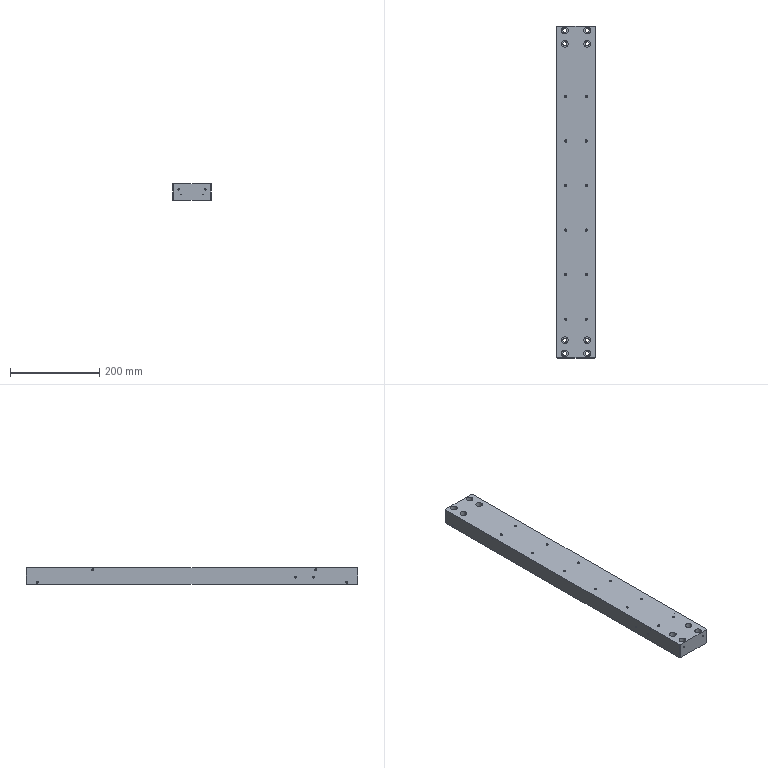Part | STEP file | Y-axis module mounting plate 590 | 1 solid | 176 faces | box 86 x 745 x 36 mm | volume 2257304 mm3 | cylinder 96 | cone 62 | plane 18 | commonest cylinder face diameters 5 x24 3.3 x16 4.2 x16 9 x16 15 x16 6.8 x8